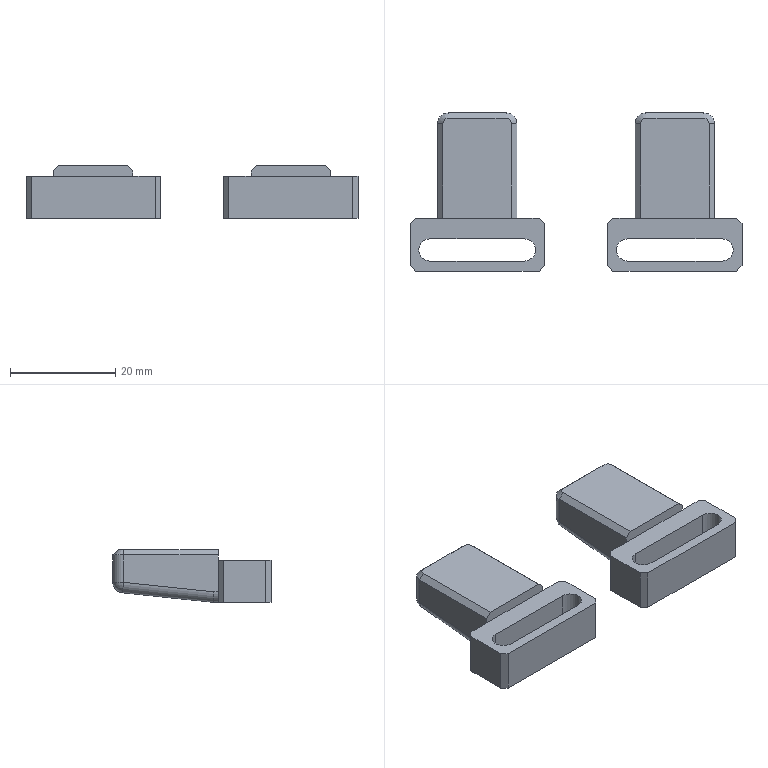NC program | NX | posted with a generic post | part box 63 x 30 x 10 mm
Lines 1 to 1609 of 2151, first 1470 of 1595 lines:
N10 G17 G21 G94 G90
(FLOOR_WALL_COPY , TOOL : D80)
N12 T19 M6
N14 G54
N16 G17 G0 G90 X-78.5 Y0. B0. C0. S6500 M3
N18 G43 Z30. H19
N20 Z3.
N22 G94 G1 Z0. F1500.
N24 X-73.5
N26 X73.5
N28 X78.5
N30 Z3.
N32 G0 Z30.
N34 M5
(ZLEVEL_PROFILE , TOOL : D10)
N36 T15 M6
N38 G54
N40 G17 G0 G90 X26.685 Y19.681 B0. C0. S9500 M3
N42 G43 Z30. H15
N44 Z1.5
N46 G94 G1 X28.002 Y19.063 Z1.424 F1000.
N48 X29.292 Y18.042 Z1.338
N50 X30.313 Y16.752 Z1.251
N52 X31.011 Y15.263 Z1.165
N54 X31.35 Y13.653 Z1.079
N56 Y0.029 Z0.365
N58 X31.896 Y-0.064 Z0.336
N60 X32.853 Y-0.441 Z0.282
N62 X33.715 Y-1.002 Z0.228
N64 X35.498 Y-2.785 Z0.096
N66 X36.24 Y-4.037 Z0.02
N68 X36.6 Y-5.446 Z-0.057
N70 Y-14.554 Z-0.534
N72 X36.24 Y-15.963 Z-0.61
N74 X35.498 Y-17.215 Z-0.686
N76 X33.715 Y-18.998 Z-0.819
N78 X32.463 Y-19.74 Z-0.895
N80 X31.054 Y-20.1 Z-0.971
N82 X30.5 Z-1.
N84 X7. F3000.
N86 G2 X3.394 Y-18.606 R5.1
N88 G1 X2.394 Y-17.606
N90 G2 X0.9 Y-14. R5.1
N92 G1 Y-6.
N94 G2 X2.394 Y-2.394 R5.1
N96 G1 X3.394 Y-1.394
N98 G2 X6.15 Y0.029 R5.1
N100 G1 Y13.
N102 G2 X13.25 Y20.1 R7.1
N104 G1 X24.25
N106 G2 X31.35 Y13. R7.1
N108 G1 Y0.029
N110 G2 X34.106 Y-1.394 R5.1
N112 G1 X35.106 Y-2.394
N114 G2 X36.6 Y-6. R5.1
N116 G1 Y-14.
N118 G2 X35.106 Y-17.606 R5.1
N120 G1 X34.106 Y-18.606
N122 G2 X30.5 Y-20.1 R5.1
N124 G1 X7.274 Z-1.405
N126 X6.887 Y-20.099 Z-1.412
N128 X6.501 Y-20.076 Z-1.419
N130 X6.118 Y-20.023 Z-1.426
N132 X5.739 Y-19.942 Z-1.432
N134 X5.368 Y-19.832 Z-1.439
N136 X5.006 Y-19.694 Z-1.446
N138 X4.656 Y-19.53 Z-1.453
N140 X4.319 Y-19.339 Z-1.459
N142 X3.998 Y-19.123 Z-1.466
N144 X3.694 Y-18.884 Z-1.473
N146 X3.409 Y-18.622 Z-1.48
N148 X3.135 Y-18.348 Z-1.486
N150 X2.588 Y-17.801 Z-1.5
N152 X2.315 Y-17.526 Z-1.507
N154 X2.058 Y-17.236 Z-1.514
N156 X1.824 Y-16.928 Z-1.52
N158 X1.614 Y-16.603 Z-1.527
N160 X1.43 Y-16.263 Z-1.534
N162 X1.271 Y-15.91 Z-1.541
N164 X1.14 Y-15.546 Z-1.547
N166 X1.037 Y-15.173 Z-1.554
N168 X0.962 Y-14.793 Z-1.561
N170 X0.916 Y-14.409 Z-1.568
N172 X0.9 Y-14.022 Z-1.574
N174 Y-13.635 Z-1.581
N176 Y-6.667 Z-1.703
N178 Y-6.28 Z-1.709
N180 X0.901 Y-5.893 Z-1.716
N182 X0.924 Y-5.507 Z-1.723
N184 X0.976 Y-5.123 Z-1.73
N186 X1.057 Y-4.745 Z-1.736
N188 X1.166 Y-4.374 Z-1.743
N190 X1.303 Y-4.012 Z-1.75
N192 X1.468 Y-3.662 Z-1.757
N194 X1.658 Y-3.325 Z-1.764
N196 X1.873 Y-3.003 Z-1.77
N198 X2.113 Y-2.699 Z-1.777
N200 X2.374 Y-2.414 Z-1.784
N202 X2.648 Y-2.14 Z-1.791
N204 X2.921 Y-1.866 Z-1.797
N206 X3.195 Y-1.592 Z-1.804
N208 X3.47 Y-1.319 Z-1.811
N210 X3.759 Y-1.062 Z-1.818
N212 X4.067 Y-0.828 Z-1.824
N214 X4.392 Y-0.617 Z-1.831
N216 X4.732 Y-0.432 Z-1.838
N218 X5.084 Y-0.273 Z-1.845
N220 X5.448 Y-0.142 Z-1.851
N222 X5.812 Y-0.04 Z-1.858
N224 X6.15 Y0.08 Z-1.865
N226 Y7.822 Z-2.
N228 Y13.
N230 G2 X13.25 Y20.1 R7.1
N232 G1 X24.25
N234 G2 X31.35 Y13. R7.1
N236 G1 Y0.029
N238 G2 X34.106 Y-1.394 R5.1
N240 G1 X35.106 Y-2.394
N242 G2 X36.6 Y-6. R5.1
N244 G1 Y-14.
N246 G2 X35.106 Y-17.606 R5.1
N248 G1 X34.106 Y-18.606
N250 G2 X30.5 Y-20.1 R5.1
N252 G1 X7.274 Z-2.405
N254 X6.887 Y-20.099 Z-2.412
N256 X6.501 Y-20.076 Z-2.419
N258 X6.118 Y-20.023 Z-2.426
N260 X5.739 Y-19.942 Z-2.432
N262 X5.368 Y-19.832 Z-2.439
N264 X5.006 Y-19.694 Z-2.446
N266 X4.656 Y-19.53 Z-2.453
N268 X4.319 Y-19.339 Z-2.459
N270 X3.998 Y-19.123 Z-2.466
N272 X3.694 Y-18.884 Z-2.473
N274 X3.409 Y-18.622 Z-2.48
N276 X3.135 Y-18.348 Z-2.486
N278 X2.588 Y-17.801 Z-2.5
N280 X2.315 Y-17.526 Z-2.507
N282 X2.058 Y-17.236 Z-2.514
N284 X1.824 Y-16.928 Z-2.52
N286 X1.614 Y-16.603 Z-2.527
N288 X1.43 Y-16.263 Z-2.534
N290 X1.271 Y-15.91 Z-2.541
N292 X1.14 Y-15.546 Z-2.547
N294 X1.037 Y-15.173 Z-2.554
N296 X0.962 Y-14.793 Z-2.561
N298 X0.916 Y-14.409 Z-2.568
N300 X0.9 Y-14.022 Z-2.574
N302 Y-13.635 Z-2.581
N304 Y-6.667 Z-2.703
N306 Y-6.28 Z-2.709
N308 X0.901 Y-5.893 Z-2.716
N310 X0.924 Y-5.507 Z-2.723
N312 X0.976 Y-5.123 Z-2.73
N314 X1.057 Y-4.745 Z-2.736
N316 X1.166 Y-4.374 Z-2.743
N318 X1.303 Y-4.012 Z-2.75
N320 X1.468 Y-3.662 Z-2.757
N322 X1.658 Y-3.325 Z-2.764
N324 X1.873 Y-3.003 Z-2.77
N326 X2.113 Y-2.699 Z-2.777
N328 X2.374 Y-2.414 Z-2.784
N330 X2.648 Y-2.14 Z-2.791
N332 X2.921 Y-1.866 Z-2.797
N334 X3.195 Y-1.592 Z-2.804
N336 X3.47 Y-1.319 Z-2.811
N338 X3.759 Y-1.062 Z-2.818
N340 X4.067 Y-0.828 Z-2.824
N342 X4.392 Y-0.617 Z-2.831
N344 X4.732 Y-0.432 Z-2.838
N346 X5.084 Y-0.273 Z-2.845
N348 X5.448 Y-0.142 Z-2.851
N350 X5.812 Y-0.04 Z-2.858
N352 X6.15 Y0.08 Z-2.865
N354 Y7.822 Z-3.
N356 Y13.
N358 G2 X13.25 Y20.1 R7.1
N360 G1 X24.25
N362 G2 X31.35 Y13. R7.1
N364 G1 Y0.029
N366 G2 X34.106 Y-1.394 R5.1
N368 G1 X35.106 Y-2.394
N370 G2 X36.6 Y-6. R5.1
N372 G1 Y-14.
N374 G2 X35.106 Y-17.606 R5.1
N376 G1 X34.106 Y-18.606
N378 G2 X30.5 Y-20.1 R5.1
N380 G1 X7.274 Z-3.405
N382 X6.887 Y-20.099 Z-3.412
N384 X6.501 Y-20.076 Z-3.419
N386 X6.118 Y-20.023 Z-3.426
N388 X5.739 Y-19.942 Z-3.432
N390 X5.368 Y-19.832 Z-3.439
N392 X5.006 Y-19.694 Z-3.446
N394 X4.656 Y-19.53 Z-3.453
N396 X4.319 Y-19.339 Z-3.459
N398 X3.998 Y-19.123 Z-3.466
N400 X3.694 Y-18.884 Z-3.473
N402 X3.409 Y-18.622 Z-3.48
N404 X3.135 Y-18.348 Z-3.486
N406 X2.588 Y-17.801 Z-3.5
N408 X2.315 Y-17.526 Z-3.507
N410 X2.058 Y-17.236 Z-3.514
N412 X1.824 Y-16.928 Z-3.52
N414 X1.614 Y-16.603 Z-3.527
N416 X1.43 Y-16.263 Z-3.534
N418 X1.271 Y-15.91 Z-3.541
N420 X1.14 Y-15.546 Z-3.547
N422 X1.037 Y-15.173 Z-3.554
N424 X0.962 Y-14.793 Z-3.561
N426 X0.916 Y-14.409 Z-3.568
N428 X0.9 Y-14.022 Z-3.574
N430 Y-13.635 Z-3.581
N432 Y-6.667 Z-3.703
N434 Y-6.28 Z-3.709
N436 X0.901 Y-5.893 Z-3.716
N438 X0.924 Y-5.507 Z-3.723
N440 X0.976 Y-5.123 Z-3.73
N442 X1.057 Y-4.745 Z-3.736
N444 X1.166 Y-4.374 Z-3.743
N446 X1.303 Y-4.012 Z-3.75
N448 X1.468 Y-3.662 Z-3.757
N450 X1.658 Y-3.325 Z-3.764
N452 X1.873 Y-3.003 Z-3.77
N454 X2.113 Y-2.699 Z-3.777
N456 X2.374 Y-2.414 Z-3.784
N458 X2.648 Y-2.14 Z-3.791
N460 X2.921 Y-1.866 Z-3.797
N462 X3.195 Y-1.592 Z-3.804
N464 X3.47 Y-1.319 Z-3.811
N466 X3.759 Y-1.062 Z-3.818
N468 X4.067 Y-0.828 Z-3.824
N470 X4.392 Y-0.617 Z-3.831
N472 X4.732 Y-0.432 Z-3.838
N474 X5.084 Y-0.273 Z-3.845
N476 X5.448 Y-0.142 Z-3.851
N478 X5.812 Y-0.04 Z-3.858
N480 X6.15 Y0.08 Z-3.865
N482 Y7.822 Z-4.
N484 Y13.
N486 G2 X13.25 Y20.1 R7.1
N488 G1 X24.25
N490 G2 X31.35 Y13. R7.1
N492 G1 Y0.029
N494 G2 X34.106 Y-1.394 R5.1
N496 G1 X35.106 Y-2.394
N498 G2 X36.6 Y-6. R5.1
N500 G1 Y-14.
N502 G2 X35.106 Y-17.606 R5.1
N504 G1 X34.106 Y-18.606
N506 G2 X30.5 Y-20.1 R5.1
N508 G1 X7.274 Z-4.405
N510 X6.887 Y-20.099 Z-4.412
N512 X6.501 Y-20.076 Z-4.419
N514 X6.118 Y-20.023 Z-4.426
N516 X5.739 Y-19.942 Z-4.432
N518 X5.368 Y-19.832 Z-4.439
N520 X5.006 Y-19.694 Z-4.446
N522 X4.656 Y-19.53 Z-4.453
N524 X4.319 Y-19.339 Z-4.459
N526 X3.998 Y-19.123 Z-4.466
N528 X3.694 Y-18.884 Z-4.473
N530 X3.409 Y-18.622 Z-4.48
N532 X3.135 Y-18.348 Z-4.486
N534 X2.588 Y-17.801 Z-4.5
N536 X2.315 Y-17.526 Z-4.507
N538 X2.058 Y-17.236 Z-4.514
N540 X1.824 Y-16.928 Z-4.52
N542 X1.614 Y-16.603 Z-4.527
N544 X1.43 Y-16.263 Z-4.534
N546 X1.271 Y-15.91 Z-4.541
N548 X1.14 Y-15.546 Z-4.547
N550 X1.037 Y-15.173 Z-4.554
N552 X0.962 Y-14.793 Z-4.561
N554 X0.916 Y-14.409 Z-4.568
N556 X0.9 Y-14.022 Z-4.574
N558 Y-13.635 Z-4.581
N560 Y-6.667 Z-4.703
N562 Y-6.28 Z-4.709
N564 X0.901 Y-5.893 Z-4.716
N566 X0.924 Y-5.507 Z-4.723
N568 X0.976 Y-5.123 Z-4.73
N570 X1.057 Y-4.745 Z-4.736
N572 X1.166 Y-4.374 Z-4.743
N574 X1.303 Y-4.012 Z-4.75
N576 X1.468 Y-3.662 Z-4.757
N578 X1.658 Y-3.325 Z-4.764
N580 X1.873 Y-3.003 Z-4.77
N582 X2.113 Y-2.699 Z-4.777
N584 X2.374 Y-2.414 Z-4.784
N586 X2.648 Y-2.14 Z-4.791
N588 X2.921 Y-1.866 Z-4.797
N590 X3.195 Y-1.592 Z-4.804
N592 X3.47 Y-1.319 Z-4.811
N594 X3.759 Y-1.062 Z-4.818
N596 X4.067 Y-0.828 Z-4.824
N598 X4.392 Y-0.617 Z-4.831
N600 X4.732 Y-0.432 Z-4.838
N602 X5.084 Y-0.273 Z-4.845
N604 X5.448 Y-0.142 Z-4.851
N606 X5.812 Y-0.04 Z-4.858
N608 X6.15 Y0.08 Z-4.865
N610 Y7.822 Z-5.
N612 Y13.
N614 G2 X13.25 Y20.1 R7.1
N616 G1 X24.25
N618 G2 X31.35 Y13. R7.1
N620 G1 Y0.029
N622 G2 X34.106 Y-1.394 R5.1
N624 G1 X35.106 Y-2.394
N626 G2 X36.6 Y-6. R5.1
N628 G1 Y-14.
N630 G2 X35.106 Y-17.606 R5.1
N632 G1 X34.106 Y-18.606
N634 G2 X30.5 Y-20.1 R5.1
N636 G1 X7.274 Z-5.405
N638 X6.887 Y-20.099 Z-5.412
N640 X6.501 Y-20.076 Z-5.419
N642 X6.118 Y-20.023 Z-5.426
N644 X5.739 Y-19.942 Z-5.432
N646 X5.368 Y-19.832 Z-5.439
N648 X5.006 Y-19.694 Z-5.446
N650 X4.656 Y-19.53 Z-5.453
N652 X4.319 Y-19.339 Z-5.459
N654 X3.998 Y-19.123 Z-5.466
N656 X3.694 Y-18.884 Z-5.473
N658 X3.409 Y-18.622 Z-5.48
N660 X3.135 Y-18.348 Z-5.486
N662 X2.588 Y-17.801 Z-5.5
N664 X2.315 Y-17.526 Z-5.507
N666 X2.058 Y-17.236 Z-5.514
N668 X1.824 Y-16.928 Z-5.52
N670 X1.614 Y-16.603 Z-5.527
N672 X1.43 Y-16.263 Z-5.534
N674 X1.271 Y-15.91 Z-5.541
N676 X1.14 Y-15.546 Z-5.547
N678 X1.037 Y-15.173 Z-5.554
N680 X0.962 Y-14.793 Z-5.561
N682 X0.916 Y-14.409 Z-5.568
N684 X0.9 Y-14.022 Z-5.574
N686 Y-13.635 Z-5.581
N688 Y-6.667 Z-5.703
N690 Y-6.28 Z-5.709
N692 X0.901 Y-5.893 Z-5.716
N694 X0.924 Y-5.507 Z-5.723
N696 X0.976 Y-5.123 Z-5.73
N698 X1.057 Y-4.745 Z-5.736
N700 X1.166 Y-4.374 Z-5.743
N702 X1.303 Y-4.012 Z-5.75
N704 X1.468 Y-3.662 Z-5.757
N706 X1.658 Y-3.325 Z-5.764
N708 X1.873 Y-3.003 Z-5.77
N710 X2.113 Y-2.699 Z-5.777
N712 X2.374 Y-2.414 Z-5.784
N714 X2.648 Y-2.14 Z-5.791
N716 X2.921 Y-1.866 Z-5.797
N718 X3.195 Y-1.592 Z-5.804
N720 X3.47 Y-1.319 Z-5.811
N722 X3.759 Y-1.062 Z-5.818
N724 X4.067 Y-0.828 Z-5.824
N726 X4.392 Y-0.617 Z-5.831
N728 X4.732 Y-0.432 Z-5.838
N730 X5.084 Y-0.273 Z-5.845
N732 X5.448 Y-0.142 Z-5.851
N734 X5.812 Y-0.04 Z-5.858
N736 X6.15 Y0.08 Z-5.865
N738 Y7.822 Z-6.
N740 Y13.
N742 G2 X13.25 Y20.1 R7.1
N744 G1 X24.25
N746 G2 X31.35 Y13. R7.1
N748 G1 Y0.029
N750 G2 X34.106 Y-1.394 R5.1
N752 G1 X35.106 Y-2.394
N754 G2 X36.6 Y-6. R5.1
N756 G1 Y-14.
N758 G2 X35.106 Y-17.606 R5.1
N760 G1 X34.106 Y-18.606
N762 G2 X30.5 Y-20.1 R5.1
N764 G1 X7.274 Z-6.405
N766 X6.887 Y-20.099 Z-6.412
N768 X6.501 Y-20.076 Z-6.419
N770 X6.118 Y-20.023 Z-6.426
N772 X5.739 Y-19.942 Z-6.432
N774 X5.368 Y-19.832 Z-6.439
N776 X5.006 Y-19.694 Z-6.446
N778 X4.656 Y-19.53 Z-6.453
N780 X4.319 Y-19.339 Z-6.459
N782 X3.998 Y-19.123 Z-6.466
N784 X3.694 Y-18.884 Z-6.473
N786 X3.409 Y-18.622 Z-6.48
N788 X3.135 Y-18.348 Z-6.486
N790 X2.588 Y-17.801 Z-6.5
N792 X2.315 Y-17.526 Z-6.507
N794 X2.058 Y-17.236 Z-6.514
N796 X1.824 Y-16.928 Z-6.52
N798 X1.614 Y-16.603 Z-6.527
N800 X1.43 Y-16.263 Z-6.534
N802 X1.271 Y-15.91 Z-6.541
N804 X1.14 Y-15.546 Z-6.547
N806 X1.037 Y-15.173 Z-6.554
N808 X0.962 Y-14.793 Z-6.561
N810 X0.916 Y-14.409 Z-6.568
N812 X0.9 Y-14.022 Z-6.574
N814 Y-13.635 Z-6.581
N816 Y-6.667 Z-6.703
N818 Y-6.28 Z-6.709
N820 X0.901 Y-5.893 Z-6.716
N822 X0.924 Y-5.507 Z-6.723
N824 X0.976 Y-5.123 Z-6.73
N826 X1.057 Y-4.745 Z-6.736
N828 X1.166 Y-4.374 Z-6.743
N830 X1.303 Y-4.012 Z-6.75
N832 X1.468 Y-3.662 Z-6.757
N834 X1.658 Y-3.325 Z-6.764
N836 X1.873 Y-3.003 Z-6.77
N838 X2.113 Y-2.699 Z-6.777
N840 X2.374 Y-2.414 Z-6.784
N842 X2.648 Y-2.14 Z-6.791
N844 X2.921 Y-1.866 Z-6.797
N846 X3.195 Y-1.592 Z-6.804
N848 X3.47 Y-1.319 Z-6.811
N850 X3.759 Y-1.062 Z-6.818
N852 X4.067 Y-0.828 Z-6.824
N854 X4.392 Y-0.617 Z-6.831
N856 X4.732 Y-0.432 Z-6.838
N858 X5.084 Y-0.273 Z-6.845
N860 X5.448 Y-0.142 Z-6.851
N862 X5.812 Y-0.04 Z-6.858
N864 X6.15 Y0.08 Z-6.865
N866 Y7.822 Z-7.
N868 Y13.
N870 G2 X13.25 Y20.1 R7.1
N872 G1 X24.25
N874 G2 X31.35 Y13. R7.1
N876 G1 Y0.029
N878 G2 X34.106 Y-1.394 R5.1
N880 G1 X35.106 Y-2.394
N882 G2 X36.6 Y-6. R5.1
N884 G1 Y-14.
N886 G2 X35.106 Y-17.606 R5.1
N888 G1 X34.106 Y-18.606
N890 G2 X30.5 Y-20.1 R5.1
N892 G1 X7.274 Z-7.405
N894 X6.887 Y-20.099 Z-7.412
N896 X6.501 Y-20.076 Z-7.419
N898 X6.118 Y-20.023 Z-7.426
N900 X5.739 Y-19.942 Z-7.432
N902 X5.368 Y-19.832 Z-7.439
N904 X5.006 Y-19.694 Z-7.446
N906 X4.656 Y-19.53 Z-7.453
N908 X4.319 Y-19.339 Z-7.459
N910 X3.998 Y-19.123 Z-7.466
N912 X3.694 Y-18.884 Z-7.473
N914 X3.409 Y-18.622 Z-7.48
N916 X3.135 Y-18.348 Z-7.486
N918 X2.588 Y-17.801 Z-7.5
N920 X2.315 Y-17.526 Z-7.507
N922 X2.058 Y-17.236 Z-7.514
N924 X1.824 Y-16.928 Z-7.52
N926 X1.614 Y-16.603 Z-7.527
N928 X1.43 Y-16.263 Z-7.534
N930 X1.271 Y-15.91 Z-7.541
N932 X1.14 Y-15.546 Z-7.547
N934 X1.037 Y-15.173 Z-7.554
N936 X0.962 Y-14.793 Z-7.561
N938 X0.916 Y-14.409 Z-7.568
N940 X0.9 Y-14.022 Z-7.574
N942 Y-13.635 Z-7.581
N944 Y-6.667 Z-7.703
N946 Y-6.28 Z-7.709
N948 X0.901 Y-5.893 Z-7.716
N950 X0.924 Y-5.507 Z-7.723
N952 X0.976 Y-5.123 Z-7.73
N954 X1.057 Y-4.745 Z-7.736
N956 X1.166 Y-4.374 Z-7.743
N958 X1.303 Y-4.012 Z-7.75
N960 X1.468 Y-3.662 Z-7.757
N962 X1.658 Y-3.325 Z-7.764
N964 X1.873 Y-3.003 Z-7.77
N966 X2.113 Y-2.699 Z-7.777
N968 X2.374 Y-2.414 Z-7.784
N970 X2.648 Y-2.14 Z-7.791
N972 X2.921 Y-1.866 Z-7.797
N974 X3.195 Y-1.592 Z-7.804
N976 X3.47 Y-1.319 Z-7.811
N978 X3.759 Y-1.062 Z-7.818
N980 X4.067 Y-0.828 Z-7.824
N982 X4.392 Y-0.617 Z-7.831
N984 X4.732 Y-0.432 Z-7.838
N986 X5.084 Y-0.273 Z-7.845
N988 X5.448 Y-0.142 Z-7.851
N990 X5.812 Y-0.04 Z-7.858
N992 X6.15 Y0.08 Z-7.865
N994 Y7.822 Z-8.
N996 Y13.
N998 G2 X13.25 Y20.1 R7.1
N1000 G1 X24.25
N1002 G2 X31.35 Y13. R7.1
N1004 G1 Y0.029
N1006 G2 X34.106 Y-1.394 R5.1
N1008 G1 X35.106 Y-2.394
N1010 G2 X36.6 Y-6. R5.1
N1012 G1 Y-14.
N1014 G2 X35.106 Y-17.606 R5.1
N1016 G1 X34.106 Y-18.606
N1018 G2 X30.5 Y-20.1 R5.1
N1020 G1 X7.274 Z-8.405
N1022 X6.887 Y-20.099 Z-8.412
N1024 X6.501 Y-20.076 Z-8.419
N1026 X6.118 Y-20.023 Z-8.426
N1028 X5.739 Y-19.942 Z-8.432
N1030 X5.368 Y-19.832 Z-8.439
N1032 X5.006 Y-19.694 Z-8.446
N1034 X4.656 Y-19.53 Z-8.453
N1036 X4.319 Y-19.339 Z-8.459
N1038 X3.998 Y-19.123 Z-8.466
N1040 X3.694 Y-18.884 Z-8.473
N1042 X3.409 Y-18.622 Z-8.48
N1044 X3.135 Y-18.348 Z-8.486
N1046 X2.588 Y-17.801 Z-8.5
N1048 X2.315 Y-17.526 Z-8.507
N1050 X2.058 Y-17.236 Z-8.514
N1052 X1.824 Y-16.928 Z-8.52
N1054 X1.614 Y-16.603 Z-8.527
N1056 X1.43 Y-16.263 Z-8.534
N1058 X1.271 Y-15.91 Z-8.541
N1060 X1.14 Y-15.546 Z-8.547
N1062 X1.037 Y-15.173 Z-8.554
N1064 X0.962 Y-14.793 Z-8.561
N1066 X0.916 Y-14.409 Z-8.568
N1068 X0.9 Y-14.022 Z-8.574
N1070 Y-13.635 Z-8.581
N1072 Y-6.667 Z-8.703
N1074 Y-6.28 Z-8.709
N1076 X0.901 Y-5.893 Z-8.716
N1078 X0.924 Y-5.507 Z-8.723
N1080 X0.976 Y-5.123 Z-8.73
N1082 X1.057 Y-4.745 Z-8.736
N1084 X1.166 Y-4.374 Z-8.743
N1086 X1.303 Y-4.012 Z-8.75
N1088 X1.468 Y-3.662 Z-8.757
N1090 X1.658 Y-3.325 Z-8.764
N1092 X1.873 Y-3.003 Z-8.77
N1094 X2.113 Y-2.699 Z-8.777
N1096 X2.374 Y-2.414 Z-8.784
N1098 X2.648 Y-2.14 Z-8.791
N1100 X2.921 Y-1.866 Z-8.797
N1102 X3.195 Y-1.592 Z-8.804
N1104 X3.47 Y-1.319 Z-8.811
N1106 X3.759 Y-1.062 Z-8.818
N1108 X4.067 Y-0.828 Z-8.824
N1110 X4.392 Y-0.617 Z-8.831
N1112 X4.732 Y-0.432 Z-8.838
N1114 X5.084 Y-0.273 Z-8.845
N1116 X5.448 Y-0.142 Z-8.851
N1118 X5.812 Y-0.04 Z-8.858
N1120 X6.15 Y0.08 Z-8.865
N1122 Y7.822 Z-9.
N1124 Y13.
N1126 G2 X13.25 Y20.1 R7.1
N1128 G1 X24.25
N1130 G2 X31.35 Y13. R7.1
N1132 G1 Y0.029
N1134 G2 X34.106 Y-1.394 R5.1
N1136 G1 X35.106 Y-2.394
N1138 G2 X36.6 Y-6. R5.1
N1140 G1 Y-14.
N1142 G2 X35.106 Y-17.606 R5.1
N1144 G1 X34.106 Y-18.606
N1146 G2 X30.5 Y-20.1 R5.1
N1148 G1 X7.274 Z-9.405
N1150 X6.887 Y-20.099 Z-9.412
N1152 X6.501 Y-20.076 Z-9.419
N1154 X6.118 Y-20.023 Z-9.426
N1156 X5.739 Y-19.942 Z-9.432
N1158 X5.368 Y-19.832 Z-9.439
N1160 X5.006 Y-19.694 Z-9.446
N1162 X4.656 Y-19.53 Z-9.453
N1164 X4.319 Y-19.339 Z-9.459
N1166 X3.998 Y-19.123 Z-9.466
N1168 X3.694 Y-18.884 Z-9.473
N1170 X3.409 Y-18.622 Z-9.48
N1172 X3.135 Y-18.348 Z-9.486
N1174 X2.588 Y-17.801 Z-9.5
N1176 X2.315 Y-17.526 Z-9.507
N1178 X2.058 Y-17.236 Z-9.514
N1180 X1.824 Y-16.928 Z-9.52
N1182 X1.614 Y-16.603 Z-9.527
N1184 X1.43 Y-16.263 Z-9.534
N1186 X1.271 Y-15.91 Z-9.541
N1188 X1.14 Y-15.546 Z-9.547
N1190 X1.037 Y-15.173 Z-9.554
N1192 X0.962 Y-14.793 Z-9.561
N1194 X0.916 Y-14.409 Z-9.568
N1196 X0.9 Y-14.022 Z-9.574
N1198 Y-13.635 Z-9.581
N1200 Y-6.667 Z-9.703
N1202 Y-6.28 Z-9.709
N1204 X0.901 Y-5.893 Z-9.716
N1206 X0.924 Y-5.507 Z-9.723
N1208 X0.976 Y-5.123 Z-9.73
N1210 X1.057 Y-4.745 Z-9.736
N1212 X1.166 Y-4.374 Z-9.743
N1214 X1.303 Y-4.012 Z-9.75
N1216 X1.468 Y-3.662 Z-9.757
N1218 X1.658 Y-3.325 Z-9.764
N1220 X1.873 Y-3.003 Z-9.77
N1222 X2.113 Y-2.699 Z-9.777
N1224 X2.374 Y-2.414 Z-9.784
N1226 X2.648 Y-2.14 Z-9.791
N1228 X2.921 Y-1.866 Z-9.797
N1230 X3.195 Y-1.592 Z-9.804
N1232 X3.47 Y-1.319 Z-9.811
N1234 X3.759 Y-1.062 Z-9.818
N1236 X4.067 Y-0.828 Z-9.824
N1238 X4.392 Y-0.617 Z-9.831
N1240 X4.732 Y-0.432 Z-9.838
N1242 X5.084 Y-0.273 Z-9.845
N1244 X5.448 Y-0.142 Z-9.851
N1246 X5.812 Y-0.04 Z-9.858
N1248 X6.15 Y0.08 Z-9.865
N1250 Y7.822 Z-10.
N1252 Y13.
N1254 G2 X13.25 Y20.1 R7.1
N1256 G1 X24.25
N1258 G2 X31.35 Y13. R7.1
N1260 G1 Y0.029
N1262 G2 X34.106 Y-1.394 R5.1
N1264 G1 X35.106 Y-2.394
N1266 G2 X36.6 Y-6. R5.1
N1268 G1 Y-14.
N1270 G2 X35.106 Y-17.606 R5.1
N1272 G1 X34.106 Y-18.606
N1274 G2 X30.5 Y-20.1 R5.1
N1276 G1 X7.
N1278 G2 X3.394 Y-18.606 R5.1
N1280 G1 X2.394 Y-17.606
N1282 G2 X0.9 Y-14. R5.1
N1284 G1 Y-6.
N1286 G2 X2.394 Y-2.394 R5.1
N1288 G1 X3.394 Y-1.394
N1290 G2 X6.15 Y0.029 R5.1
N1292 G1 Y7.822
N1294 Z-8.5
N1296 G0 Z53.
N1298 X-10.815 Y19.681
N1300 Z1.5
N1302 G1 X-9.498 Y19.063 Z1.424 F1000.
N1304 X-8.208 Y18.042 Z1.338
N1306 X-7.187 Y16.752 Z1.251
N1308 X-6.489 Y15.263 Z1.165
N1310 X-6.15 Y13.653 Z1.079
N1312 Y0.029 Z0.365
N1314 X-5.604 Y-0.064 Z0.336
N1316 X-4.647 Y-0.441 Z0.282
N1318 X-3.785 Y-1.002 Z0.228
N1320 X-2.002 Y-2.785 Z0.096
N1322 X-1.26 Y-4.037 Z0.02
N1324 X-0.9 Y-5.446 Z-0.057
N1326 Y-14.554 Z-0.534
N1328 X-1.26 Y-15.963 Z-0.61
N1330 X-2.002 Y-17.215 Z-0.686
N1332 X-3.785 Y-18.998 Z-0.819
N1334 X-5.037 Y-19.74 Z-0.895
N1336 X-6.446 Y-20.1 Z-0.971
N1338 X-7. Z-1.
N1340 X-30.5 F3000.
N1342 G2 X-34.106 Y-18.606 R5.1
N1344 G1 X-35.106 Y-17.606
N1346 G2 X-36.6 Y-14. R5.1
N1348 G1 Y-6.
N1350 G2 X-35.106 Y-2.394 R5.1
N1352 G1 X-34.106 Y-1.394
N1354 G2 X-31.35 Y0.029 R5.1
N1356 G1 Y13.
N1358 G2 X-24.25 Y20.1 R7.1
N1360 G1 X-13.25
N1362 G2 X-6.15 Y13. R7.1
N1364 G1 Y0.029
N1366 G2 X-3.394 Y-1.394 R5.1
N1368 G1 X-2.394 Y-2.394
N1370 G2 X-0.9 Y-6. R5.1
N1372 G1 Y-14.
N1374 G2 X-2.394 Y-17.606 R5.1
N1376 G1 X-3.394 Y-18.606
N1378 G2 X-7. Y-20.1 R5.1
N1380 G1 X-30.226 Z-1.405
N1382 X-30.613 Y-20.099 Z-1.412
N1384 X-30.999 Y-20.076 Z-1.419
N1386 X-31.382 Y-20.023 Z-1.426
N1388 X-31.761 Y-19.942 Z-1.432
N1390 X-32.132 Y-19.832 Z-1.439
N1392 X-32.494 Y-19.694 Z-1.446
N1394 X-32.844 Y-19.53 Z-1.453
N1396 X-33.181 Y-19.339 Z-1.459
N1398 X-33.502 Y-19.123 Z-1.466
N1400 X-33.806 Y-18.884 Z-1.473
N1402 X-34.091 Y-18.622 Z-1.48
N1404 X-34.365 Y-18.348 Z-1.486
N1406 X-34.912 Y-17.801 Z-1.5
N1408 X-35.185 Y-17.526 Z-1.507
N1410 X-35.442 Y-17.236 Z-1.514
N1412 X-35.676 Y-16.928 Z-1.52
N1414 X-35.886 Y-16.603 Z-1.527
N1416 X-36.07 Y-16.263 Z-1.534
N1418 X-36.229 Y-15.91 Z-1.541
N1420 X-36.36 Y-15.546 Z-1.547
N1422 X-36.463 Y-15.173 Z-1.554
N1424 X-36.538 Y-14.793 Z-1.561
N1426 X-36.584 Y-14.409 Z-1.568
N1428 X-36.6 Y-14.022 Z-1.574
N1430 Y-13.635 Z-1.581
N1432 Y-6.667 Z-1.703
N1434 Y-6.28 Z-1.709
N1436 X-36.599 Y-5.893 Z-1.716
N1438 X-36.576 Y-5.507 Z-1.723
N1440 X-36.524 Y-5.123 Z-1.73
N1442 X-36.443 Y-4.745 Z-1.736
N1444 X-36.334 Y-4.374 Z-1.743
N1446 X-36.197 Y-4.012 Z-1.75
N1448 X-36.032 Y-3.662 Z-1.757
N1450 X-35.842 Y-3.325 Z-1.764
N1452 X-35.627 Y-3.003 Z-1.77
N1454 X-35.387 Y-2.699 Z-1.777
N1456 X-35.126 Y-2.414 Z-1.784
N1458 X-34.852 Y-2.14 Z-1.791
N1460 X-34.579 Y-1.866 Z-1.797
N1462 X-34.305 Y-1.592 Z-1.804
N1464 X-34.03 Y-1.319 Z-1.811
N1466 X-33.741 Y-1.062 Z-1.818
N1468 X-33.433 Y-0.828 Z-1.824
N1470 X-33.108 Y-0.617 Z-1.831
N1472 X-32.768 Y-0.432 Z-1.838
N1474 X-32.416 Y-0.273 Z-1.845
N1476 X-32.052 Y-0.142 Z-1.851
N1478 X-31.688 Y-0.04 Z-1.858
N1480 X-31.35 Y0.08 Z-1.865
N1482 Y7.822 Z-2.
N1484 Y13.
N1486 G2 X-24.25 Y20.1 R7.1
N1488 G1 X-13.25
N1490 G2 X-6.15 Y13. R7.1
N1492 G1 Y0.029
N1494 G2 X-3.394 Y-1.394 R5.1
N1496 G1 X-2.394 Y-2.394
N1498 G2 X-0.9 Y-6. R5.1
N1500 G1 Y-14.
N1502 G2 X-2.394 Y-17.606 R5.1
N1504 G1 X-3.394 Y-18.606
N1506 G2 X-7. Y-20.1 R5.1
N1508 G1 X-30.226 Z-2.405
N1510 X-30.613 Y-20.099 Z-2.412
N1512 X-30.999 Y-20.076 Z-2.419
N1514 X-31.382 Y-20.023 Z-2.426
N1516 X-31.761 Y-19.942 Z-2.432
N1518 X-32.132 Y-19.832 Z-2.439
N1520 X-32.494 Y-19.694 Z-2.446
N1522 X-32.844 Y-19.53 Z-2.453
N1524 X-33.181 Y-19.339 Z-2.459
N1526 X-33.502 Y-19.123 Z-2.466
N1528 X-33.806 Y-18.884 Z-2.473
N1530 X-34.091 Y-18.622 Z-2.48
N1532 X-34.365 Y-18.348 Z-2.486
N1534 X-34.912 Y-17.801 Z-2.5
N1536 X-35.185 Y-17.526 Z-2.507
N1538 X-35.442 Y-17.236 Z-2.514
N1540 X-35.676 Y-16.928 Z-2.52
N1542 X-35.886 Y-16.603 Z-2.527
N1544 X-36.07 Y-16.263 Z-2.534
N1546 X-36.229 Y-15.91 Z-2.541
N1548 X-36.36 Y-15.546 Z-2.547
N1550 X-36.463 Y-15.173 Z-2.554
N1552 X-36.538 Y-14.793 Z-2.561
N1554 X-36.584 Y-14.409 Z-2.568
N1556 X-36.6 Y-14.022 Z-2.574
N1558 Y-13.635 Z-2.581
N1560 Y-6.667 Z-2.703
N1562 Y-6.28 Z-2.709
N1564 X-36.599 Y-5.893 Z-2.716
N1566 X-36.576 Y-5.507 Z-2.723
N1568 X-36.524 Y-5.123 Z-2.73
N1570 X-36.443 Y-4.745 Z-2.736
N1572 X-36.334 Y-4.374 Z-2.743
N1574 X-36.197 Y-4.012 Z-2.75
N1576 X-36.032 Y-3.662 Z-2.757
N1578 X-35.842 Y-3.325 Z-2.764
N1580 X-35.627 Y-3.003 Z-2.77
N1582 X-35.387 Y-2.699 Z-2.777
N1584 X-35.126 Y-2.414 Z-2.784
N1586 X-34.852 Y-2.14 Z-2.791
N1588 X-34.579 Y-1.866 Z-2.797
N1590 X-34.305 Y-1.592 Z-2.804
N1592 X-34.03 Y-1.319 Z-2.811
N1594 X-33.741 Y-1.062 Z-2.818
N1596 X-33.433 Y-0.828 Z-2.824
N1598 X-33.108 Y-0.617 Z-2.831
N1600 X-32.768 Y-0.432 Z-2.838
N1602 X-32.416 Y-0.273 Z-2.845
N1604 X-32.052 Y-0.142 Z-2.851
N1606 X-31.688 Y-0.04 Z-2.858
N1608 X-31.35 Y0.08 Z-2.865
N1610 Y7.822 Z-3.
N1612 Y13.
N1614 G2 X-24.25 Y20.1 R7.1
N1616 G1 X-13.25
N1618 G2 X-6.15 Y13. R7.1
N1620 G1 Y0.029
N1622 G2 X-3.394 Y-1.394 R5.1
N1624 G1 X-2.394 Y-2.394
N1626 G2 X-0.9 Y-6. R5.1
N1628 G1 Y-14.
N1630 G2 X-2.394 Y-17.606 R5.1
N1632 G1 X-3.394 Y-18.606
N1634 G2 X-7. Y-20.1 R5.1
N1636 G1 X-30.226 Z-3.405
N1638 X-30.613 Y-20.099 Z-3.412
N1640 X-30.999 Y-20.076 Z-3.419
N1642 X-31.382 Y-20.023 Z-3.426
N1644 X-31.761 Y-19.942 Z-3.432
N1646 X-32.132 Y-19.832 Z-3.439
N1648 X-32.494 Y-19.694 Z-3.446
N1650 X-32.844 Y-19.53 Z-3.453
N1652 X-33.181 Y-19.339 Z-3.459
N1654 X-33.502 Y-19.123 Z-3.466
N1656 X-33.806 Y-18.884 Z-3.473
N1658 X-34.091 Y-18.622 Z-3.48
N1660 X-34.365 Y-18.348 Z-3.486
N1662 X-34.912 Y-17.801 Z-3.5
N1664 X-35.185 Y-17.526 Z-3.507
N1666 X-35.442 Y-17.236 Z-3.514
N1668 X-35.676 Y-16.928 Z-3.52
N1670 X-35.886 Y-16.603 Z-3.527
N1672 X-36.07 Y-16.263 Z-3.534
N1674 X-36.229 Y-15.91 Z-3.541
N1676 X-36.36 Y-15.546 Z-3.547
N1678 X-36.463 Y-15.173 Z-3.554
N1680 X-36.538 Y-14.793 Z-3.561
N1682 X-36.584 Y-14.409 Z-3.568
N1684 X-36.6 Y-14.022 Z-3.574
N1686 Y-13.635 Z-3.581
N1688 Y-6.667 Z-3.703
N1690 Y-6.28 Z-3.709
N1692 X-36.599 Y-5.893 Z-3.716
N1694 X-36.576 Y-5.507 Z-3.723
N1696 X-36.524 Y-5.123 Z-3.73
N1698 X-36.443 Y-4.745 Z-3.736
N1700 X-36.334 Y-4.374 Z-3.743
N1702 X-36.197 Y-4.012 Z-3.75
N1704 X-36.032 Y-3.662 Z-3.757
N1706 X-35.842 Y-3.325 Z-3.764
N1708 X-35.627 Y-3.003 Z-3.77
N1710 X-35.387 Y-2.699 Z-3.777
N1712 X-35.126 Y-2.414 Z-3.784
N1714 X-34.852 Y-2.14 Z-3.791
N1716 X-34.579 Y-1.866 Z-3.797
N1718 X-34.305 Y-1.592 Z-3.804
N1720 X-34.03 Y-1.319 Z-3.811
N1722 X-33.741 Y-1.062 Z-3.818
N1724 X-33.433 Y-0.828 Z-3.824
N1726 X-33.108 Y-0.617 Z-3.831
N1728 X-32.768 Y-0.432 Z-3.838
N1730 X-32.416 Y-0.273 Z-3.845
N1732 X-32.052 Y-0.142 Z-3.851
N1734 X-31.688 Y-0.04 Z-3.858
N1736 X-31.35 Y0.08 Z-3.865
N1738 Y7.822 Z-4.
N1740 Y13.
N1742 G2 X-24.25 Y20.1 R7.1
N1744 G1 X-13.25
N1746 G2 X-6.15 Y13. R7.1
N1748 G1 Y0.029
N1750 G2 X-3.394 Y-1.394 R5.1
N1752 G1 X-2.394 Y-2.394
N1754 G2 X-0.9 Y-6. R5.1
N1756 G1 Y-14.
N1758 G2 X-2.394 Y-17.606 R5.1
N1760 G1 X-3.394 Y-18.606
N1762 G2 X-7. Y-20.1 R5.1
N1764 G1 X-30.226 Z-4.405
N1766 X-30.613 Y-20.099 Z-4.412
N1768 X-30.999 Y-20.076 Z-4.419
N1770 X-31.382 Y-20.023 Z-4.426
N1772 X-31.761 Y-19.942 Z-4.432
N1774 X-32.132 Y-19.832 Z-4.439
N1776 X-32.494 Y-19.694 Z-4.446
N1778 X-32.844 Y-19.53 Z-4.453
N1780 X-33.181 Y-19.339 Z-4.459
N1782 X-33.502 Y-19.123 Z-4.466
N1784 X-33.806 Y-18.884 Z-4.473
N1786 X-34.091 Y-18.622 Z-4.48
N1788 X-34.365 Y-18.348 Z-4.486
N1790 X-34.912 Y-17.801 Z-4.5
N1792 X-35.185 Y-17.526 Z-4.507
N1794 X-35.442 Y-17.236 Z-4.514
N1796 X-35.676 Y-16.928 Z-4.52
N1798 X-35.886 Y-16.603 Z-4.527
N1800 X-36.07 Y-16.263 Z-4.534
N1802 X-36.229 Y-15.91 Z-4.541
N1804 X-36.36 Y-15.546 Z-4.547
N1806 X-36.463 Y-15.173 Z-4.554
N1808 X-36.538 Y-14.793 Z-4.561
N1810 X-36.584 Y-14.409 Z-4.568
N1812 X-36.6 Y-14.022 Z-4.574
N1814 Y-13.635 Z-4.581
N1816 Y-6.667 Z-4.703
N1818 Y-6.28 Z-4.709
N1820 X-36.599 Y-5.893 Z-4.716
N1822 X-36.576 Y-5.507 Z-4.723
N1824 X-36.524 Y-5.123 Z-4.73
N1826 X-36.443 Y-4.745 Z-4.736
N1828 X-36.334 Y-4.374 Z-4.743
N1830 X-36.197 Y-4.012 Z-4.75
N1832 X-36.032 Y-3.662 Z-4.757
N1834 X-35.842 Y-3.325 Z-4.764
N1836 X-35.627 Y-3.003 Z-4.77
N1838 X-35.387 Y-2.699 Z-4.777
N1840 X-35.126 Y-2.414 Z-4.784
N1842 X-34.852 Y-2.14 Z-4.791
N1844 X-34.579 Y-1.866 Z-4.797
N1846 X-34.305 Y-1.592 Z-4.804
N1848 X-34.03 Y-1.319 Z-4.811
N1850 X-33.741 Y-1.062 Z-4.818
N1852 X-33.433 Y-0.828 Z-4.824
N1854 X-33.108 Y-0.617 Z-4.831
N1856 X-32.768 Y-0.432 Z-4.838
N1858 X-32.416 Y-0.273 Z-4.845
N1860 X-32.052 Y-0.142 Z-4.851
N1862 X-31.688 Y-0.04 Z-4.858
N1864 X-31.35 Y0.08 Z-4.865
N1866 Y7.822 Z-5.
N1868 Y13.
N1870 G2 X-24.25 Y20.1 R7.1
N1872 G1 X-13.25
N1874 G2 X-6.15 Y13. R7.1
N1876 G1 Y0.029
N1878 G2 X-3.394 Y-1.394 R5.1
N1880 G1 X-2.394 Y-2.394
N1882 G2 X-0.9 Y-6. R5.1
N1884 G1 Y-14.
N1886 G2 X-2.394 Y-17.606 R5.1
N1888 G1 X-3.394 Y-18.606
N1890 G2 X-7. Y-20.1 R5.1
N1892 G1 X-30.226 Z-5.405
N1894 X-30.613 Y-20.099 Z-5.412
N1896 X-30.999 Y-20.076 Z-5.419
N1898 X-31.382 Y-20.023 Z-5.426
N1900 X-31.761 Y-19.942 Z-5.432
N1902 X-32.132 Y-19.832 Z-5.439
N1904 X-32.494 Y-19.694 Z-5.446
N1906 X-32.844 Y-19.53 Z-5.453
N1908 X-33.181 Y-19.339 Z-5.459
N1910 X-33.502 Y-19.123 Z-5.466
N1912 X-33.806 Y-18.884 Z-5.473
N1914 X-34.091 Y-18.622 Z-5.48
N1916 X-34.365 Y-18.348 Z-5.486
N1918 X-34.912 Y-17.801 Z-5.5
N1920 X-35.185 Y-17.526 Z-5.507
N1922 X-35.442 Y-17.236 Z-5.514
N1924 X-35.676 Y-16.928 Z-5.52
N1926 X-35.886 Y-16.603 Z-5.527
N1928 X-36.07 Y-16.263 Z-5.534
N1930 X-36.229 Y-15.91 Z-5.541
N1932 X-36.36 Y-15.546 Z-5.547
N1934 X-36.463 Y-15.173 Z-5.554
N1936 X-36.538 Y-14.793 Z-5.561
N1938 X-36.584 Y-14.409 Z-5.568
N1940 X-36.6 Y-14.022 Z-5.574
N1942 Y-13.635 Z-5.581
N1944 Y-6.667 Z-5.703
N1946 Y-6.28 Z-5.709
N1948 X-36.599 Y-5.893 Z-5.716
N1950 X-36.576 Y-5.507 Z-5.723
N1952 X-36.524 Y-5.123 Z-5.73
N1954 X-36.443 Y-4.745 Z-5.736
N1956 X-36.334 Y-4.374 Z-5.743
N1958 X-36.197 Y-4.012 Z-5.75
N1960 X-36.032 Y-3.662 Z-5.757
N1962 X-35.842 Y-3.325 Z-5.764
N1964 X-35.627 Y-3.003 Z-5.77
N1966 X-35.387 Y-2.699 Z-5.777
N1968 X-35.126 Y-2.414 Z-5.784
N1970 X-34.852 Y-2.14 Z-5.791
N1972 X-34.579 Y-1.866 Z-5.797
N1974 X-34.305 Y-1.592 Z-5.804
N1976 X-34.03 Y-1.319 Z-5.811
N1978 X-33.741 Y-1.062 Z-5.818
N1980 X-33.433 Y-0.828 Z-5.824
N1982 X-33.108 Y-0.617 Z-5.831
N1984 X-32.768 Y-0.432 Z-5.838
N1986 X-32.416 Y-0.273 Z-5.845
N1988 X-32.052 Y-0.142 Z-5.851
N1990 X-31.688 Y-0.04 Z-5.858
N1992 X-31.35 Y0.08 Z-5.865
N1994 Y7.822 Z-6.
N1996 Y13.
N1998 G2 X-24.25 Y20.1 R7.1
N2000 G1 X-13.25
N2002 G2 X-6.15 Y13. R7.1
N2004 G1 Y0.029
N2006 G2 X-3.394 Y-1.394 R5.1
N2008 G1 X-2.394 Y-2.394
N2010 G2 X-0.9 Y-6. R5.1
N2012 G1 Y-14.
N2014 G2 X-2.394 Y-17.606 R5.1
N2016 G1 X-3.394 Y-18.606
N2018 G2 X-7. Y-20.1 R5.1
N2020 G1 X-30.226 Z-6.405
N2022 X-30.613 Y-20.099 Z-6.412
N2024 X-30.999 Y-20.076 Z-6.419
N2026 X-31.382 Y-20.023 Z-6.426
N2028 X-31.761 Y-19.942 Z-6.432
N2030 X-32.132 Y-19.832 Z-6.439
N2032 X-32.494 Y-19.694 Z-6.446
N2034 X-32.844 Y-19.53 Z-6.453
N2036 X-33.181 Y-19.339 Z-6.459
N2038 X-33.502 Y-19.123 Z-6.466
N2040 X-33.806 Y-18.884 Z-6.473
N2042 X-34.091 Y-18.622 Z-6.48
N2044 X-34.365 Y-18.348 Z-6.486
N2046 X-34.912 Y-17.801 Z-6.5
N2048 X-35.185 Y-17.526 Z-6.507
N2050 X-35.442 Y-17.236 Z-6.514
N2052 X-35.676 Y-16.928 Z-6.52
N2054 X-35.886 Y-16.603 Z-6.527
N2056 X-36.07 Y-16.263 Z-6.534
N2058 X-36.229 Y-15.91 Z-6.541
N2060 X-36.36 Y-15.546 Z-6.547
N2062 X-36.463 Y-15.173 Z-6.554
N2064 X-36.538 Y-14.793 Z-6.561
N2066 X-36.584 Y-14.409 Z-6.568
N2068 X-36.6 Y-14.022 Z-6.574
N2070 Y-13.635 Z-6.581
N2072 Y-6.667 Z-6.703
N2074 Y-6.28 Z-6.709
N2076 X-36.599 Y-5.893 Z-6.716
N2078 X-36.576 Y-5.507 Z-6.723
N2080 X-36.524 Y-5.123 Z-6.73
N2082 X-36.443 Y-4.745 Z-6.736
N2084 X-36.334 Y-4.374 Z-6.743
N2086 X-36.197 Y-4.012 Z-6.75
N2088 X-36.032 Y-3.662 Z-6.757
N2090 X-35.842 Y-3.325 Z-6.764
N2092 X-35.627 Y-3.003 Z-6.77
N2094 X-35.387 Y-2.699 Z-6.777
N2096 X-35.126 Y-2.414 Z-6.784
N2098 X-34.852 Y-2.14 Z-6.791
N2100 X-34.579 Y-1.866 Z-6.797
N2102 X-34.305 Y-1.592 Z-6.804
N2104 X-34.03 Y-1.319 Z-6.811
N2106 X-33.741 Y-1.062 Z-6.818
N2108 X-33.433 Y-0.828 Z-6.824
N2110 X-33.108 Y-0.617 Z-6.831
N2112 X-32.768 Y-0.432 Z-6.838
N2114 X-32.416 Y-0.273 Z-6.845
N2116 X-32.052 Y-0.142 Z-6.851
N2118 X-31.688 Y-0.04 Z-6.858
N2120 X-31.35 Y0.08 Z-6.865
N2122 Y7.822 Z-7.
N2124 Y13.
N2126 G2 X-24.25 Y20.1 R7.1
N2128 G1 X-13.25
N2130 G2 X-6.15 Y13. R7.1
N2132 G1 Y0.029
N2134 G2 X-3.394 Y-1.394 R5.1
N2136 G1 X-2.394 Y-2.394
N2138 G2 X-0.9 Y-6. R5.1
N2140 G1 Y-14.
N2142 G2 X-2.394 Y-17.606 R5.1
N2144 G1 X-3.394 Y-18.606
N2146 G2 X-7. Y-20.1 R5.1
N2148 G1 X-30.226 Z-7.405
N2150 X-30.613 Y-20.099 Z-7.412
N2152 X-30.999 Y-20.076 Z-7.419
N2154 X-31.382 Y-20.023 Z-7.426
N2156 X-31.761 Y-19.942 Z-7.432
N2158 X-32.132 Y-19.832 Z-7.439
N2160 X-32.494 Y-19.694 Z-7.446
N2162 X-32.844 Y-19.53 Z-7.453
N2164 X-33.181 Y-19.339 Z-7.459
N2166 X-33.502 Y-19.123 Z-7.466
N2168 X-33.806 Y-18.884 Z-7.473
N2170 X-34.091 Y-18.622 Z-7.48
N2172 X-34.365 Y-18.348 Z-7.486
N2174 X-34.912 Y-17.801 Z-7.5
N2176 X-35.185 Y-17.526 Z-7.507
N2178 X-35.442 Y-17.236 Z-7.514
N2180 X-35.676 Y-16.928 Z-7.52
N2182 X-35.886 Y-16.603 Z-7.527
N2184 X-36.07 Y-16.263 Z-7.534
N2186 X-36.229 Y-15.91 Z-7.541
N2188 X-36.36 Y-15.546 Z-7.547
N2190 X-36.463 Y-15.173 Z-7.554
N2192 X-36.538 Y-14.793 Z-7.561
N2194 X-36.584 Y-14.409 Z-7.568
N2196 X-36.6 Y-14.022 Z-7.574
N2198 Y-13.635 Z-7.581
N2200 Y-6.667 Z-7.703
N2202 Y-6.28 Z-7.709
N2204 X-36.599 Y-5.893 Z-7.716
N2206 X-36.576 Y-5.507 Z-7.723
N2208 X-36.524 Y-5.123 Z-7.73
N2210 X-36.443 Y-4.745 Z-7.736
N2212 X-36.334 Y-4.374 Z-7.743
N2214 X-36.197 Y-4.012 Z-7.75
N2216 X-36.032 Y-3.662 Z-7.757
N2218 X-35.842 Y-3.325 Z-7.764
N2220 X-35.627 Y-3.003 Z-7.77
N2222 X-35.387 Y-2.699 Z-7.777
N2224 X-35.126 Y-2.414 Z-7.784
N2226 X-34.852 Y-2.14 Z-7.791
N2228 X-34.579 Y-1.866 Z-7.797
N2230 X-34.305 Y-1.592 Z-7.804
N2232 X-34.03 Y-1.319 Z-7.811
N2234 X-33.741 Y-1.062 Z-7.818
N2236 X-33.433 Y-0.828 Z-7.824
N2238 X-33.108 Y-0.617 Z-7.831
N2240 X-32.768 Y-0.432 Z-7.838
N2242 X-32.416 Y-0.273 Z-7.845
N2244 X-32.052 Y-0.142 Z-7.851
N2246 X-31.688 Y-0.04 Z-7.858
N2248 X-31.35 Y0.08 Z-7.865
N2250 Y7.822 Z-8.
N2252 Y13.
N2254 G2 X-24.25 Y20.1 R7.1
N2256 G1 X-13.25
N2258 G2 X-6.15 Y13. R7.1
N2260 G1 Y0.029
N2262 G2 X-3.394 Y-1.394 R5.1
N2264 G1 X-2.394 Y-2.394
N2266 G2 X-0.9 Y-6. R5.1
N2268 G1 Y-14.
N2270 G2 X-2.394 Y-17.606 R5.1
N2272 G1 X-3.394 Y-18.606
N2274 G2 X-7. Y-20.1 R5.1
N2276 G1 X-30.226 Z-8.405
N2278 X-30.613 Y-20.099 Z-8.412
N2280 X-30.999 Y-20.076 Z-8.419
N2282 X-31.382 Y-20.023 Z-8.426
N2284 X-31.761 Y-19.942 Z-8.432
N2286 X-32.132 Y-19.832 Z-8.439
N2288 X-32.494 Y-19.694 Z-8.446
N2290 X-32.844 Y-19.53 Z-8.453
N2292 X-33.181 Y-19.339 Z-8.459
N2294 X-33.502 Y-19.123 Z-8.466
N2296 X-33.806 Y-18.884 Z-8.473
N2298 X-34.091 Y-18.622 Z-8.48
N2300 X-34.365 Y-18.348 Z-8.486
N2302 X-34.912 Y-17.801 Z-8.5
N2304 X-35.185 Y-17.526 Z-8.507
N2306 X-35.442 Y-17.236 Z-8.514
N2308 X-35.676 Y-16.928 Z-8.52
N2310 X-35.886 Y-16.603 Z-8.527
N2312 X-36.07 Y-16.263 Z-8.534
N2314 X-36.229 Y-15.91 Z-8.541
N2316 X-36.36 Y-15.546 Z-8.547
N2318 X-36.463 Y-15.173 Z-8.554
N2320 X-36.538 Y-14.793 Z-8.561
N2322 X-36.584 Y-14.409 Z-8.568
N2324 X-36.6 Y-14.022 Z-8.574
N2326 Y-13.635 Z-8.581
N2328 Y-6.667 Z-8.703
N2330 Y-6.28 Z-8.709
N2332 X-36.599 Y-5.893 Z-8.716
N2334 X-36.576 Y-5.507 Z-8.723
N2336 X-36.524 Y-5.123 Z-8.73
N2338 X-36.443 Y-4.745 Z-8.736
N2340 X-36.334 Y-4.374 Z-8.743
N2342 X-36.197 Y-4.012 Z-8.75
N2344 X-36.032 Y-3.662 Z-8.757
N2346 X-35.842 Y-3.325 Z-8.764
N2348 X-35.627 Y-3.003 Z-8.77
N2350 X-35.387 Y-2.699 Z-8.777
N2352 X-35.126 Y-2.414 Z-8.784
N2354 X-34.852 Y-2.14 Z-8.791
N2356 X-34.579 Y-1.866 Z-8.797
N2358 X-34.305 Y-1.592 Z-8.804
N2360 X-34.03 Y-1.319 Z-8.811
N2362 X-33.741 Y-1.062 Z-8.818
N2364 X-33.433 Y-0.828 Z-8.824
N2366 X-33.108 Y-0.617 Z-8.831
N2368 X-32.768 Y-0.432 Z-8.838
N2370 X-32.416 Y-0.273 Z-8.845
N2372 X-32.052 Y-0.142 Z-8.851
N2374 X-31.688 Y-0.04 Z-8.858
N2376 X-31.35 Y0.08 Z-8.865
N2378 Y7.822 Z-9.
N2380 Y13.
N2382 G2 X-24.25 Y20.1 R7.1
N2384 G1 X-13.25
N2386 G2 X-6.15 Y13. R7.1
N2388 G1 Y0.029
N2390 G2 X-3.394 Y-1.394 R5.1
N2392 G1 X-2.394 Y-2.394
N2394 G2 X-0.9 Y-6. R5.1
N2396 G1 Y-14.
N2398 G2 X-2.394 Y-17.606 R5.1
N2400 G1 X-3.394 Y-18.606
N2402 G2 X-7. Y-20.1 R5.1
N2404 G1 X-30.226 Z-9.405
N2406 X-30.613 Y-20.099 Z-9.412
N2408 X-30.999 Y-20.076 Z-9.419
N2410 X-31.382 Y-20.023 Z-9.426
N2412 X-31.761 Y-19.942 Z-9.432
N2414 X-32.132 Y-19.832 Z-9.439
N2416 X-32.494 Y-19.694 Z-9.446
N2418 X-32.844 Y-19.53 Z-9.453
N2420 X-33.181 Y-19.339 Z-9.459
N2422 X-33.502 Y-19.123 Z-9.466
N2424 X-33.806 Y-18.884 Z-9.473
N2426 X-34.091 Y-18.622 Z-9.48
N2428 X-34.365 Y-18.348 Z-9.486
N2430 X-34.912 Y-17.801 Z-9.5
N2432 X-35.185 Y-17.526 Z-9.507
N2434 X-35.442 Y-17.236 Z-9.514
N2436 X-35.676 Y-16.928 Z-9.52
N2438 X-35.886 Y-16.603 Z-9.527
N2440 X-36.07 Y-16.263 Z-9.534
N2442 X-36.229 Y-15.91 Z-9.541
N2444 X-36.36 Y-15.546 Z-9.547
N2446 X-36.463 Y-15.173 Z-9.554
N2448 X-36.538 Y-14.793 Z-9.561
N2450 X-36.584 Y-14.409 Z-9.568
N2452 X-36.6 Y-14.022 Z-9.574
N2454 Y-13.635 Z-9.581
N2456 Y-6.667 Z-9.703
N2458 Y-6.28 Z-9.709
N2460 X-36.599 Y-5.893 Z-9.716
N2462 X-36.576 Y-5.507 Z-9.723
N2464 X-36.524 Y-5.123 Z-9.73
N2466 X-36.443 Y-4.745 Z-9.736
N2468 X-36.334 Y-4.374 Z-9.743
N2470 X-36.197 Y-4.012 Z-9.75
N2472 X-36.032 Y-3.662 Z-9.757
N2474 X-35.842 Y-3.325 Z-9.764
N2476 X-35.627 Y-3.003 Z-9.77
N2478 X-35.387 Y-2.699 Z-9.777
N2480 X-35.126 Y-2.414 Z-9.784
N2482 X-34.852 Y-2.14 Z-9.791
N2484 X-34.579 Y-1.866 Z-9.797
N2486 X-34.305 Y-1.592 Z-9.804
N2488 X-34.03 Y-1.319 Z-9.811
N2490 X-33.741 Y-1.062 Z-9.818
N2492 X-33.433 Y-0.828 Z-9.824
N2494 X-33.108 Y-0.617 Z-9.831
N2496 X-32.768 Y-0.432 Z-9.838
N2498 X-32.416 Y-0.273 Z-9.845
N2500 X-32.052 Y-0.142 Z-9.851
N2502 X-31.688 Y-0.04 Z-9.858
N2504 X-31.35 Y0.08 Z-9.865
N2506 Y7.822 Z-10.
N2508 Y13.
N2510 G2 X-24.25 Y20.1 R7.1
N2512 G1 X-13.25
N2514 G2 X-6.15 Y13. R7.1
N2516 G1 Y0.029
N2518 G2 X-3.394 Y-1.394 R5.1
N2520 G1 X-2.394 Y-2.394
N2522 G2 X-0.9 Y-6. R5.1
N2524 G1 Y-14.
N2526 G2 X-2.394 Y-17.606 R5.1
N2528 G1 X-3.394 Y-18.606
N2530 G2 X-7. Y-20.1 R5.1
N2532 G1 X-30.5
N2534 G2 X-34.106 Y-18.606 R5.1
N2536 G1 X-35.106 Y-17.606
N2538 G2 X-36.6 Y-14. R5.1
N2540 G1 Y-6.
N2542 G2 X-35.106 Y-2.394 R5.1
N2544 G1 X-34.106 Y-1.394
N2546 G2 X-31.35 Y0.029 R5.1
N2548 G1 Y7.822
N2550 Z-8.5
N2552 G0 Z30.
(FLOOR_WALL , TOOL : D10)
N2554 X-17.307 Y-21.5
N2556 Z0.05
N2558 G1 Z-0.95 F1000.
N2560 X-17.884 Y-20.5
N2562 G3 X-18.75 Y-20. R1.
N2564 G1 X-32.571 F2500.
N2566 X-36.5 Y-16.071
N2568 Y-3.929
N2570 X-32.571 Y0.
N2572 X-31.35
N2574 Y-10.1
N2576 X-6.15
N2578 Y0.
N2580 X-4.929
N2582 X-1. Y-3.929
N2584 Y-16.071
N2586 X-4.929 Y-20.
N2588 X-18.75
N2590 Y-15.5
N2592 X-30.707
N2594 X-31.615 Y-14.592
N2596 G3 X-31.35 Y-14.6 R4.5
N2598 G1 X-6.15
N2600 G3 X-5.885 Y-14.592 R4.5
N2602 G1 X-6.793 Y-15.5
N2604 X-18.75
N2606 G3 X-19.616 Y-16. R1.
N2608 G1 Z0.05
N2610 G0 X-17.307 Y-21.5 Z-0.9
N2612 G1 Z-1.9 F1000.
N2614 X-17.884 Y-20.5
N2616 G3 X-18.75 Y-20. R1.
N2618 G1 X-32.571 F2500.
N2620 X-36.5 Y-16.071
N2622 Y-3.929
N2624 X-32.571 Y0.
N2626 X-31.35
N2628 Y-10.1
N2630 X-6.15
N2632 Y0.
N2634 X-4.929
N2636 X-1. Y-3.929
N2638 Y-16.071
N2640 X-4.929 Y-20.
N2642 X-18.75
N2644 Y-15.5
N2646 X-30.707
N2648 X-31.615 Y-14.592
N2650 G3 X-31.35 Y-14.6 R4.5
N2652 G1 X-6.15
N2654 G3 X-5.885 Y-14.592 R4.5
N2656 G1 X-6.793 Y-15.5
N2658 X-18.75
N2660 G3 X-19.616 Y-16. R1.
N2662 G1 Z-0.9
N2664 G0 Z30.
N2666 X20.193 Y-21.5
N2668 Z0.05
N2670 G1 Z-0.95 F1000.
N2672 X19.616 Y-20.5
N2674 G3 X18.75 Y-20. R1.
N2676 G1 X4.929 F2500.
N2678 X1. Y-16.071
N2680 Y-3.929
N2682 X4.929 Y0.
N2684 X6.15
N2686 Y-10.1
N2688 X31.35
N2690 Y0.
N2692 X32.571
N2694 X36.5 Y-3.929
N2696 Y-16.071
N2698 X32.571 Y-20.
N2700 X18.75
N2702 Y-15.5
N2704 X6.793
N2706 X5.885 Y-14.592
N2708 G3 X6.15 Y-14.6 R4.5
N2710 G1 X31.35
N2712 G3 X31.615 Y-14.592 R4.5
N2714 G1 X30.707 Y-15.5
N2716 X18.75
N2718 G3 X17.884 Y-16. R1.
N2720 G1 Z0.05
N2722 G0 X20.193 Y-21.5 Z-0.9
N2724 G1 Z-1.9 F1000.
N2726 X19.616 Y-20.5
N2728 G3 X18.75 Y-20. R1.
N2730 G1 X4.929 F2500.
N2732 X1. Y-16.071
N2734 Y-3.929
N2736 X4.929 Y0.
N2738 X6.15
N2740 Y-10.1
N2742 X31.35
N2744 Y0.
N2746 X32.571
N2748 X36.5 Y-3.929
N2750 Y-16.071
N2752 X32.571 Y-20.
N2754 X18.75
N2756 Y-15.5
N2758 X6.793
N2760 X5.885 Y-14.592
N2762 G3 X6.15 Y-14.6 R4.5
N2764 G1 X31.35
N2766 G3 X31.615 Y-14.592 R4.5
N2768 G1 X30.707 Y-15.5
N2770 X18.75
N2772 G3 X17.884 Y-16. R1.
N2774 G1 Z-0.9
N2776 G0 Z30.
(PLANAR_PROFILE , TOOL : D10)
N2778 X0.25 Y-13.
N2780 Z2.
N2782 G1 Z-1. F1000.
N2784 Y-5.
N2786 Y13. F2500.
N2788 Y21.
N2790 Z2.
N2792 G0 Z1.
N2794 G1 Z-2. F1000.
N2796 Y13.
N2798 Y-5. F2500.
N2800 Y-13.
N2802 Z1.
N2804 G0 Z0.
N2806 G1 Z-3. F1000.
N2808 Y-5.
N2810 Y13. F2500.
N2812 Y21.
N2814 Z0.
N2816 G0 Z-1.
N2818 G1 Z-4. F1000.
N2820 Y13.
N2822 Y-5. F2500.
N2824 Y-13.
N2826 Z-1.
N2828 G0 Z-2.
N2830 G1 Z-5. F1000.
N2832 Y-5.
N2834 Y13. F2500.
N2836 Y21.
N2838 Z-2.
N2840 G0 Z-3.
N2842 G1 Z-6. F1000.
N2844 Y13.
N2846 Y-5. F2500.
N2848 Y-13.
N2850 Z-3.
N2852 G0 Z-4.
N2854 G1 Z-7. F1000.
N2856 Y-5.
N2858 Y13. F2500.
N2860 Y21.
N2862 Z-4.
N2864 G0 Z-5.
N2866 G1 Z-8. F1000.
N2868 Y13.
N2870 Y-5. F2500.
N2872 Y-13.
N2874 Z-5.
N2876 G0 Z-6.
N2878 G1 Z-9. F1000.
N2880 Y-5.
N2882 Y13. F2500.
N2884 Y21.
N2886 Z-6.
N2888 G0 Z-7.
N2890 G1 Z-10. F1000.
N2892 Y13.
N2894 Y-5. F2500.
N2896 Y-13.
N2898 Z-7.
N2900 G0 Z30.
N2902 M5
(ZLEVEL_PROFILE_COPY_1_COPY_COPY_1 , TOOL : D10JING)
N2904 T14 M6
N2906 G54
N2908 G17 G0 G90 X32.122 Y-21.809 B0. C0. S9500 M3
N2910 G43 Z30. H14
N2912 Z-9.
N2914 G94 G1 Z-10. F1000.
N2916 X31.366 Y-20.5
N2918 G3 X30.5 Y-20. R1.
N2920 G1 X7. F1200.
N2922 G2 X3.464 Y-18.536 R5.
N2924 G1 X2.464 Y-17.536
N2926 G2 X1. Y-14. R5.
N2928 G1 Y-6.
N2930 G2 X2.464 Y-2.464 R5.
N2932 G1 X3.464 Y-1.464
N2934 G2 X6.25 Y-0.057 R5.
N2936 G1 Y13.
N2938 G2 X13.25 Y20. R7.